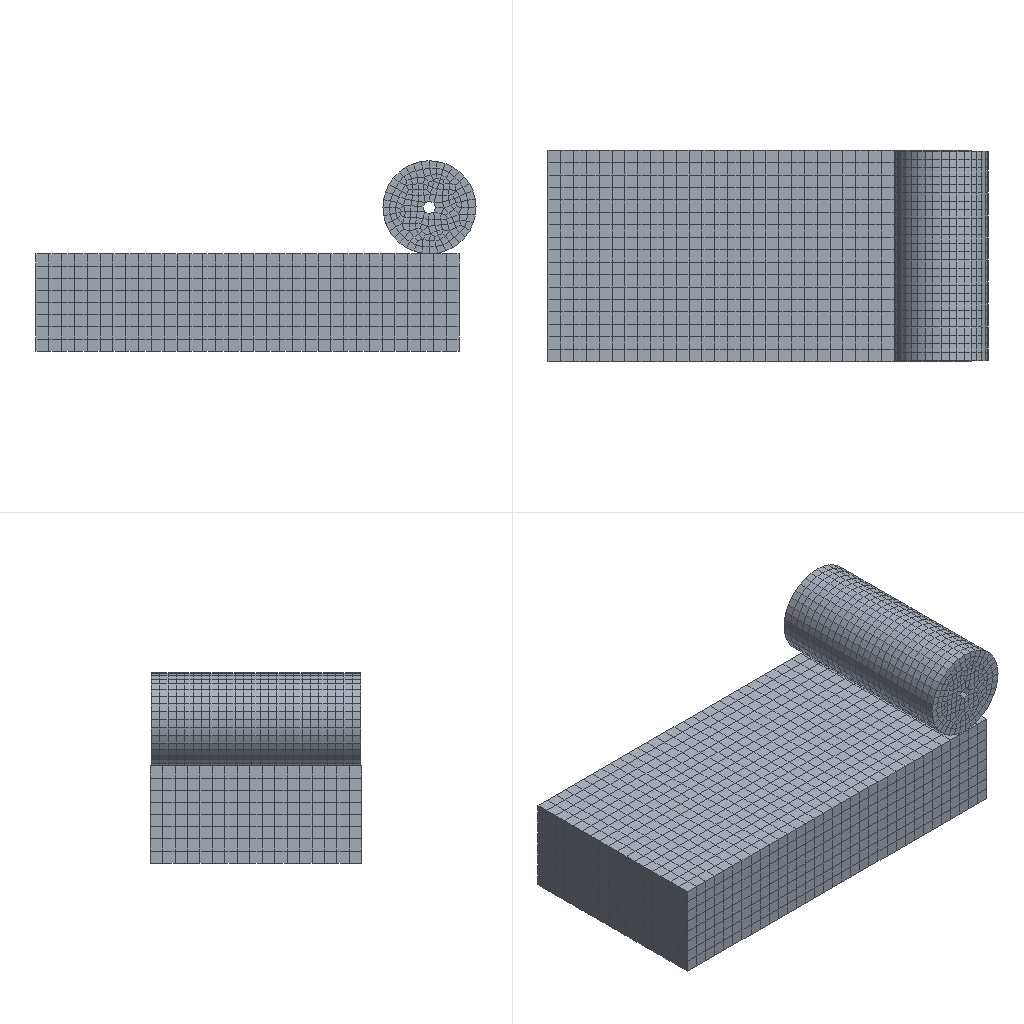Simulation study | abaqus
Set-up summary:
category,name,step,type,value,unit,region
solver,abaqus
solver,version,,,Abaqus/Standard 2020
units,not stated in the deck,,not stated
analysis,deck,,coupled temperature-displacement,coupled temperature-displacement
load_step,Step-1,Step-1,coupled temperature-displacement
load_step,requested,,,1
mesh,nodes,,,10604
mesh,elements,,,8838
element_type,C3D8RT,,solid,8838
load,load commands in deck,,count,2
bc,support commands in deck,,count,10
material,MATERIAL-1,,in results
check,setup vs results,,match,"per instance, exact: element labels, types and connectivity; labels of the nodes the elements use; coordinates of those nodes at SINGLE_PRECISION in 2 of 2 instance(s)"
Abaqus input file, long lists of numbers shortened:
*Heading
** Job name: Job-2 Model name: Model-1-Copy
** Generated by: Abaqus/CAE 2020
*Preprint, echo=NO, model=NO, history=NO, contact=NO
**
** PARTS
**
*Part, name=ban
*Node
      1,        -500.,        -500.,         230.
      2,        -500.,  -470.588,         230.
** (5506 more lines like these left out)
*Element, type=C3D8RT
   1,  163,  164,  182,  181,    1,    2,   20,   19
   2,  164,  165,  183,  182,    2,    3,   21,   20
** (4486 more lines like these left out)
*Nset, nset=Set-1, generate
    1,  5508,     1
*Elset, elset=Set-1, generate
    1,  4488,     1
** Section: Section-1
*Solid Section, elset=Set-1, material=Material-1
,
*End Part
**
*Part, name=gun
*Node
      1,   14.982, -0.7376,           0.
      2,   11.115,   10.072,           0.
** (5094 more lines like these left out)
*Element, type=C3D8RT
   1,  333,  286,  249,  299,  137,   90,   53,  103
   2,  242,  258,  197,  198,   46,   62,    1,    2
** (4348 more lines like these left out)
*Nset, nset=Set-3, generate
    1,  5096,     1
*Elset, elset=Set-3, generate
    1,  4350,     1
** Section: Section-1
*Solid Section, elset=Set-3, material=Material-1
,
*End Part
**
**
** ASSEMBLY
**
*Assembly, name=Assembly
**
*Instance, name=ban-1, part=ban
       -430.,           0.,        -345.
*End Instance
**
*Instance, name=gun-1, part=gun
          0.,         -2.5,          -5.
          0.,         -2.5,          -5., 1.,         -2.5,          -5., 90.
*End Instance
**
*Node
      1,           0.,        -250.,          -5.
*Nset, nset=Set-1, instance=gun-1
    1,    2,    3,    4,    5,    6,    7,    8,  197,  198,  199,  200,  201,  202,  203,  204
  393,  394,  395,  396,  397,  398,  399,  400,  589,  590,  591,  592,  593,  594,  595,  596
** (11 more lines like these left out)
*Elset, elset=Set-1, instance=gun-1
    2,    5,    6,   15,   19,   27,   31,   42,  176,  179,  180,  189,  193,  201,  205,  216
  350,  353,  354,  363,  367,  375,  379,  390,  524,  527,  528,  537,  541,  549,  553,  564
** (11 more lines like these left out)
*Nset, nset=Set-2, instance=ban-1
    1,    2,    3,    4,    5,    6,    7,    8,    9,   10,   11,   12,   13,   14,   15,   16
   17,   18,   19,   20,   21,   22,   23,   24,   25,   26,   27,   28,   29,   30,   31,   32
** (55 more lines like these left out)
*Elset, elset=Set-2, instance=ban-1
    1,    2,    3,    4,    5,    6,    7,    8,    9,   10,   11,   12,   13,   14,   15,   16
   17,   18,   19,   20,   21,   22,   23,   24,   25,   26,   27,   28,   29,   30,   31,   32
** (46 more lines like these left out)
*Nset, nset=Set-3, instance=ban-1, generate
   1,  162,    1
*Elset, elset=Set-3, instance=ban-1, generate
   1,  136,    1
*Nset, nset=Set-4, instance=gun-1
    1,    2,    3,    4,    5,    6,    7,    8,    9,   10,   11,   12,   13,   14,   15,   16
   17,   18,   19,   20,   21,   22,   23,   24,   25,   26,   27,   28,   29,   30,   31,   32
** (23 more lines like these left out)
*Elset, elset=Set-4, instance=gun-1
    1,    2,    3,    4,    5,    6,    7,    8,    9,   10,   11,   12,   13,   14,   15,   16
   17,   18,   19,   20,   21,   22,   23,   24,   25,   26,   27,   28,   29,   30,   31,   32
** (20 more lines like these left out)
*Nset, nset=Set-5, instance=gun-1
    1,    2,    3,    4,    5,    6,    7,    8,  197,  198,  199,  200,  201,  202,  203,  204
  393,  394,  395,  396,  397,  398,  399,  400,  589,  590,  591,  592,  593,  594,  595,  596
** (11 more lines like these left out)
*Elset, elset=Set-5, instance=gun-1
    2,    5,    6,   15,   19,   27,   31,   42,  176,  179,  180,  189,  193,  201,  205,  216
  350,  353,  354,  363,  367,  375,  379,  390,  524,  527,  528,  537,  541,  549,  553,  564
** (11 more lines like these left out)
*Nset, nset=Set-7
 1,
*Nset, nset=Set-8, instance=ban-1
  145,  146,  147,  148,  149,  150,  151,  152,  153,  154,  155,  156,  157,  158,  159,  160
  161,  162,  307,  308,  309,  310,  311,  312,  313,  314,  315,  316,  317,  318,  319,  320
** (37 more lines like these left out)
*Elset, elset=Set-8, instance=ban-1
  120,  121,  122,  123,  124,  125,  126,  127,  128,  129,  130,  131,  132,  133,  134,  135
  136,  256,  257,  258,  259,  260,  261,  262,  263,  264,  265,  266,  267,  268,  269,  270
** (34 more lines like these left out)
*Nset, nset=Set-9
 1,
*Nset, nset=Set-10, instance=ban-1
  145,  146,  147,  148,  149,  150,  151,  152,  153,  154,  155,  156,  157,  158,  159,  160
  161,  162,  307,  308,  309,  310,  311,  312,  313,  314,  315,  316,  317,  318,  319,  320
** (37 more lines like these left out)
*Elset, elset=Set-10, instance=ban-1
  120,  121,  122,  123,  124,  125,  126,  127,  128,  129,  130,  131,  132,  133,  134,  135
  136,  256,  257,  258,  259,  260,  261,  262,  263,  264,  265,  266,  267,  268,  269,  270
** (34 more lines like these left out)
*Nset, nset=m_Set-6
 1,
*Elset, elset=_Surf-1_S5, internal, instance=ban-1
  120,  121,  122,  123,  124,  125,  126,  127,  128,  129,  130,  131,  132,  133,  134,  135
  136,  256,  257,  258,  259,  260,  261,  262,  263,  264,  265,  266,  267,  268,  269,  270
** (34 more lines like these left out)
*Surface, type=ELEMENT, name=Surf-1
_Surf-1_S5, S5
*Elset, elset=_m_Surf-2_S3, internal, instance=ban-1
    1,    2,    3,    4,    5,    6,    7,    8,    9,   10,   11,   12,   13,   14,   15,   16
   17,  137,  138,  139,  140,  141,  142,  143,  144,  145,  146,  147,  148,  149,  150,  151
** (34 more lines like these left out)
*Surface, type=ELEMENT, name=m_Surf-2
_m_Surf-2_S3, S3
*Elset, elset=_s_Surf-2_S5, internal, instance=gun-1
   10,   12,   14,   16,   18,   23,   29,   30,   33,   34,   38,   39,   41,   43,   46,   65
   67,   75,   78,   83,  184,  186,  188,  190,  192,  197,  203,  204,  207,  208,  212,  213
** (30 more lines like these left out)
*Elset, elset=_s_Surf-2_S3, internal, instance=gun-1
   25,   28,   32,   36,   40,   51,   53,   54,   56,   57,   58,   70,   76,   80,   84,   85
  199,  202,  206,  210,  214,  225,  227,  228,  230,  231,  232,  244,  250,  254,  258,  259
** (23 more lines like these left out)
*Surface, type=ELEMENT, name=s_Surf-2
_s_Surf-2_S5, S5
_s_Surf-2_S3, S3
*Elset, elset=_s_Surf-4_S5, internal, instance=gun-1
    2,    6,   27,  176,  180,  201,  350,  354,  375,  524,  528,  549,  698,  702,  723,  872
  876,  897, 1046, 1050, 1071, 1220, 1224, 1245, 1394, 1398, 1419, 1568, 1572, 1593, 1742, 1746
** (3 more lines like these left out)
*Elset, elset=_s_Surf-4_S6, internal, instance=gun-1
    5,   15,  179,  189,  353,  363,  527,  537,  701,  711,  875,  885, 1049, 1059, 1223, 1233
 1397, 1407, 1571, 1581, 1745, 1755, 1919, 1929, 2093, 2103, 2267, 2277, 2441, 2451, 2615, 2625
** (2 more lines like these left out)
*Elset, elset=_s_Surf-4_S3, internal, instance=gun-1, generate
   19,  4195,   174
*Elset, elset=_s_Surf-4_S4, internal, instance=gun-1
   31,   42,  205,  216,  379,  390,  553,  564,  727,  738,  901,  912, 1075, 1086, 1249, 1260
 1423, 1434, 1597, 1608, 1771, 1782, 1945, 1956, 2119, 2130, 2293, 2304, 2467, 2478, 2641, 2652
** (2 more lines like these left out)
*Surface, type=ELEMENT, name=s_Surf-4
_s_Surf-4_S5, S5
_s_Surf-4_S6, S6
_s_Surf-4_S4, S4
_s_Surf-4_S3, S3
** Constraint: Constraint-1
*Coupling, constraint name=Constraint-1, ref node=m_Set-6, surface=s_Surf-4
*Kinematic
*End Assembly
*Amplitude, name=Amp-1
             0.,              0.,              1.,              1.
**
** MATERIALS
**
*Material, name=Material-1
*Conductivity
30.,
*Density
 2.6e-09,
*Elastic
72000., 0.3
*Expansion
 1e-06,
*Specific Heat
 4e+08,
**
** INTERACTION PROPERTIES
**
*Surface Interaction, name=IntProp-1
1.,
*Friction, slip tolerance=0.005
 0.5,
*Surface Behavior, pressure-overclosure=HARD
*Gap Conductance
 0.8,    0.
  0., 0.001
**
** INTERACTIONS
**
** Interaction: Int-1
*Contact Pair, interaction=IntProp-1, type=SURFACE TO SURFACE
m_Surf-2, s_Surf-2
** ----------------------------------------------------------------
**
** STEP: Step-1
**
*Step, name=Step-1, nlgeom=YES
*Coupled Temperature-displacement, creep=none, deltmx=1e+10, stabilize=0.0002, allsdtol=0.05, continue=NO
0.01, 5., 5e-05, 5.
**
** BOUNDARY CONDITIONS
**
** Name: BC-1 Type: 位移/转角
*Boundary
Set-7, 1, 1
Set-7, 2, 2
Set-7, 4, 4
Set-7, 6, 6
** Name: BC-2 Type: 位移/转角
*Boundary
Set-10, 2, 2
Set-10, 3, 3
Set-10, 4, 4
Set-10, 5, 5
Set-10, 6, 6
** Name: BC-3 Type: 位移/转角
*Boundary, amplitude=Amp-1
Set-3, 1, 1, 900.
**
** LOADS
**
** Name: Load-2   Type: Concentrated force
*Cload
Set-9, 3, -10000.
**
** OUTPUT REQUESTS
**
*Restart, write, number interval=1, time marks=NO
**
** FIELD OUTPUT: F-Output-1
**
*Output, field
*Node Output
CF, NT, RF, RFL, RM, RT, U, V
*Element Output, directions=YES
E, HFL, LE, MISES, MISESMAX, MISESONLY, PE, PEEQ, PEEQMAX, PEEQT, PEMAG, S, SF, SSAVG, TEMP, TSHR
VEEQ, YIELDPOT
*Contact Output
CDISP, CSTRESS
**
** HISTORY OUTPUT: H-Output-1
**
*Output, history, variable=PRESELECT
*End Step
Results summary:
result,step,,partial,increments=18 time=0.03197/5.0
result,analysis,,,"coupled temperature-displacement, steady state"
result,last_loadstep,,,1
result,primary field,,,"U, NT11"
result,reaction total,,FX,0.000803,model units
result,reaction total,,FY,4e-06,model units
result,reaction total,,FZ,10000,model units